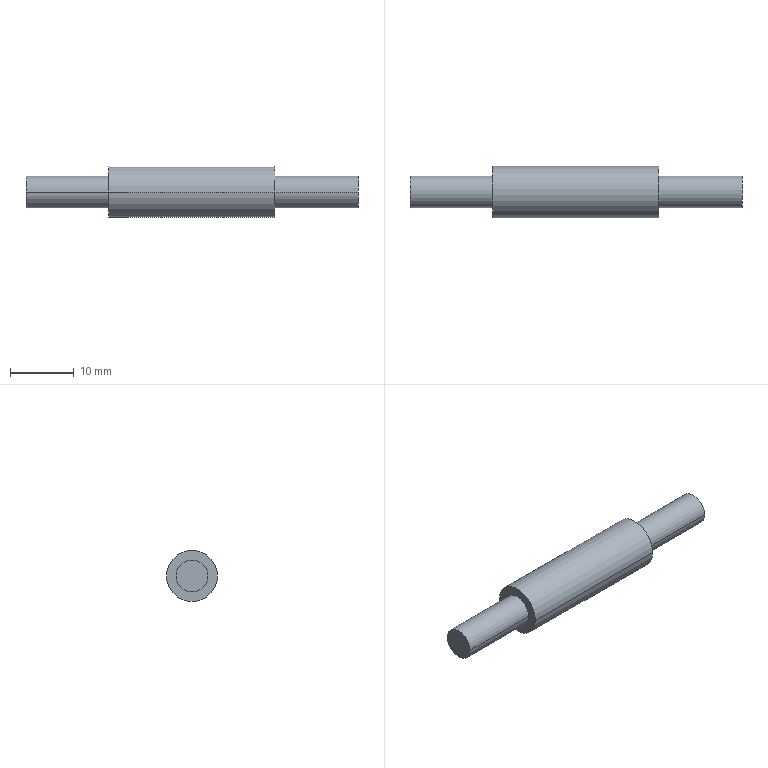Part | SolidWorks | features Revolution 1 | 1 solid | 10 faces | box 52 x 8 x 8 mm | volume 1817 mm3 | cylinder 6 | plane 4 | commonest cylinder face diameters 5 x4 8 x2
STEP:
#1=CARTESIAN_POINT('',(13.,2.5,0.));
#2=VERTEX_POINT('',#1);
#3=CARTESIAN_POINT('',(13.,-2.5,0.));
#4=VERTEX_POINT('',#3);
#5=CARTESIAN_POINT('',(13.,0.,0.));
#6=DIRECTION('',(1.,0.,0.));
#7=DIRECTION('',(0.,1.,0.));
#8=AXIS2_PLACEMENT_3D('',#5,#6,#7);
#9=CIRCLE('',#8,2.5);
#10=EDGE_CURVE('',#2,#4,#9,.T.);
#11=ORIENTED_EDGE('',*,*,#10,.T.);
#12=CARTESIAN_POINT('',(26.,-2.5,0.));
#13=VERTEX_POINT('',#12);
#14=CARTESIAN_POINT('',(26.,-2.5,0.));
#15=DIRECTION('',(1.,0.,0.));
#16=VECTOR('',#15,1000.);
#17=LINE('',#14,#16);
#18=EDGE_CURVE('',#4,#13,#17,.T.);
#19=ORIENTED_EDGE('',*,*,#18,.T.);
#20=CARTESIAN_POINT('',(26.,2.5,0.));
#21=VERTEX_POINT('',#20);
#22=CARTESIAN_POINT('',(26.,0.,0.));
#23=DIRECTION('',(1.,0.,0.));
#24=DIRECTION('',(0.,1.,0.));
#25=AXIS2_PLACEMENT_3D('',#22,#23,#24);
#26=CIRCLE('',#25,2.5);
#27=EDGE_CURVE('',#21,#13,#26,.T.);
#28=ORIENTED_EDGE('',*,*,#27,.F.);
#29=CARTESIAN_POINT('',(26.,2.5,0.));
#30=DIRECTION('',(1.,0.,0.));
#31=VECTOR('',#30,1000.);
#32=LINE('',#29,#31);
#33=EDGE_CURVE('',#2,#21,#32,.T.);
#34=ORIENTED_EDGE('',*,*,#33,.F.);
#35=EDGE_LOOP('',(#11,#19,#28,#34));
#36=FACE_OUTER_BOUND('',#35,.T.);
#37=CARTESIAN_POINT('',(26.,0.,0.));
#38=DIRECTION('',(1.,0.,0.));
#39=DIRECTION('',(0.,1.,0.));
#40=AXIS2_PLACEMENT_3D('',#37,#38,#39);
#41=CYLINDRICAL_SURFACE('',#40,2.5);
#42=ADVANCED_FACE('',(#36),#41,.T.);
#43=CARTESIAN_POINT('',(-13.,4.,0.));
#44=VERTEX_POINT('',#43);
#45=CARTESIAN_POINT('',(-13.,-4.,0.));
#46=VERTEX_POINT('',#45);
#47=CARTESIAN_POINT('',(-13.,0.,0.));
#48=DIRECTION('',(1.,0.,0.));
#49=DIRECTION('',(0.,1.,0.));
#50=AXIS2_PLACEMENT_3D('',#47,#48,#49);
#51=CIRCLE('',#50,4.);
#52=EDGE_CURVE('',#44,#46,#51,.T.);
#53=ORIENTED_EDGE('',*,*,#52,.T.);
#54=CARTESIAN_POINT('',(13.,-4.,0.));
#55=VERTEX_POINT('',#54);
#56=CARTESIAN_POINT('',(26.,-4.,0.));
#57=DIRECTION('',(1.,0.,0.));
#58=VECTOR('',#57,1000.);
#59=LINE('',#56,#58);
#60=EDGE_CURVE('',#46,#55,#59,.T.);
#61=ORIENTED_EDGE('',*,*,#60,.T.);
#62=CARTESIAN_POINT('',(13.,4.,0.));
#63=VERTEX_POINT('',#62);
#64=CARTESIAN_POINT('',(13.,0.,0.));
#65=DIRECTION('',(1.,0.,0.));
#66=DIRECTION('',(0.,1.,0.));
#67=AXIS2_PLACEMENT_3D('',#64,#65,#66);
#68=CIRCLE('',#67,4.);
#69=EDGE_CURVE('',#63,#55,#68,.T.);
#70=ORIENTED_EDGE('',*,*,#69,.F.);
#71=CARTESIAN_POINT('',(26.,4.,0.));
#72=DIRECTION('',(1.,0.,0.));
#73=VECTOR('',#72,1000.);
#74=LINE('',#71,#73);
#75=EDGE_CURVE('',#44,#63,#74,.T.);
#76=ORIENTED_EDGE('',*,*,#75,.F.);
#77=EDGE_LOOP('',(#53,#61,#70,#76));
#78=FACE_OUTER_BOUND('',#77,.T.);
#79=CARTESIAN_POINT('',(26.,0.,0.));
#80=DIRECTION('',(1.,0.,0.));
#81=DIRECTION('',(0.,1.,0.));
#82=AXIS2_PLACEMENT_3D('',#79,#80,#81);
#83=CYLINDRICAL_SURFACE('',#82,4.);
#84=ADVANCED_FACE('',(#78),#83,.T.);
#85=CARTESIAN_POINT('',(-26.,2.5,0.));
#86=VERTEX_POINT('',#85);
#87=CARTESIAN_POINT('',(-26.,-2.5,0.));
#88=VERTEX_POINT('',#87);
#89=CARTESIAN_POINT('',(-26.,0.,0.));
#90=DIRECTION('',(1.,0.,0.));
#91=DIRECTION('',(0.,1.,0.));
#92=AXIS2_PLACEMENT_3D('',#89,#90,#91);
#93=CIRCLE('',#92,2.5);
#94=EDGE_CURVE('',#86,#88,#93,.T.);
#95=ORIENTED_EDGE('',*,*,#94,.T.);
#96=CARTESIAN_POINT('',(-13.,-2.5,0.));
#97=VERTEX_POINT('',#96);
#98=CARTESIAN_POINT('',(26.,-2.5,0.));
#99=DIRECTION('',(1.,0.,0.));
#100=VECTOR('',#99,1000.);
#101=LINE('',#98,#100);
#102=EDGE_CURVE('',#88,#97,#101,.T.);
#103=ORIENTED_EDGE('',*,*,#102,.T.);
#104=CARTESIAN_POINT('',(-13.,2.5,0.));
#105=VERTEX_POINT('',#104);
#106=CARTESIAN_POINT('',(-13.,0.,0.));
#107=DIRECTION('',(1.,0.,0.));
#108=DIRECTION('',(0.,1.,0.));
#109=AXIS2_PLACEMENT_3D('',#106,#107,#108);
#110=CIRCLE('',#109,2.5);
#111=EDGE_CURVE('',#105,#97,#110,.T.);
#112=ORIENTED_EDGE('',*,*,#111,.F.);
#113=CARTESIAN_POINT('',(26.,2.5,0.));
#114=DIRECTION('',(1.,0.,0.));
#115=VECTOR('',#114,1000.);
#116=LINE('',#113,#115);
#117=EDGE_CURVE('',#86,#105,#116,.T.);
#118=ORIENTED_EDGE('',*,*,#117,.F.);
#119=EDGE_LOOP('',(#95,#103,#112,#118));
#120=FACE_OUTER_BOUND('',#119,.T.);
#121=CARTESIAN_POINT('',(26.,0.,0.));
#122=DIRECTION('',(1.,0.,0.));
#123=DIRECTION('',(0.,1.,0.));
#124=AXIS2_PLACEMENT_3D('',#121,#122,#123);
#125=CYLINDRICAL_SURFACE('',#124,2.5);
#126=ADVANCED_FACE('',(#120),#125,.T.);
#127=ORIENTED_EDGE('',*,*,#27,.T.);
#128=CARTESIAN_POINT('',(26.,0.,0.));
#129=DIRECTION('',(1.,0.,0.));
#130=DIRECTION('',(0.,1.,0.));
#131=AXIS2_PLACEMENT_3D('',#128,#129,#130);
#132=CIRCLE('',#131,2.5);
#133=EDGE_CURVE('',#13,#21,#132,.T.);
#134=ORIENTED_EDGE('',*,*,#133,.T.);
#135=EDGE_LOOP('',(#127,#134));
#136=FACE_OUTER_BOUND('',#135,.T.);
#137=CARTESIAN_POINT('',(26.,2.5,0.));
#138=DIRECTION('',(1.,0.,0.));
#139=DIRECTION('',(0.,1.,0.));
#140=AXIS2_PLACEMENT_3D('',#137,#138,#139);
#141=PLANE('',#140);
#142=ADVANCED_FACE('',(#136),#141,.T.);
#143=ORIENTED_EDGE('',*,*,#94,.F.);
#144=CARTESIAN_POINT('',(-26.,0.,0.));
#145=DIRECTION('',(1.,0.,0.));
#146=DIRECTION('',(0.,1.,0.));
#147=AXIS2_PLACEMENT_3D('',#144,#145,#146);
#148=CIRCLE('',#147,2.5);
#149=EDGE_CURVE('',#88,#86,#148,.T.);
#150=ORIENTED_EDGE('',*,*,#149,.F.);
#151=EDGE_LOOP('',(#143,#150));
#152=FACE_OUTER_BOUND('',#151,.T.);
#153=CARTESIAN_POINT('',(-26.,0.,0.));
#154=DIRECTION('',(-1.,0.,0.));
#155=DIRECTION('',(0.,-1.,0.));
#156=AXIS2_PLACEMENT_3D('',#153,#154,#155);
#157=PLANE('',#156);
#158=ADVANCED_FACE('',(#152),#157,.T.);
#159=ORIENTED_EDGE('',*,*,#102,.F.);
#160=ORIENTED_EDGE('',*,*,#149,.T.);
#161=ORIENTED_EDGE('',*,*,#117,.T.);
#162=CARTESIAN_POINT('',(-13.,0.,0.));
#163=DIRECTION('',(1.,0.,0.));
#164=DIRECTION('',(0.,1.,0.));
#165=AXIS2_PLACEMENT_3D('',#162,#163,#164);
#166=CIRCLE('',#165,2.5);
#167=EDGE_CURVE('',#97,#105,#166,.T.);
#168=ORIENTED_EDGE('',*,*,#167,.F.);
#169=EDGE_LOOP('',(#159,#160,#161,#168));
#170=FACE_OUTER_BOUND('',#169,.T.);
#171=CARTESIAN_POINT('',(26.,0.,0.));
#172=DIRECTION('',(1.,0.,0.));
#173=DIRECTION('',(0.,1.,0.));
#174=AXIS2_PLACEMENT_3D('',#171,#172,#173);
#175=CYLINDRICAL_SURFACE('',#174,2.5);
#176=ADVANCED_FACE('',(#170),#175,.T.);
#177=ORIENTED_EDGE('',*,*,#111,.T.);
#178=ORIENTED_EDGE('',*,*,#167,.T.);
#179=EDGE_LOOP('',(#177,#178));
#180=FACE_BOUND('',#179,.T.);
#181=ORIENTED_EDGE('',*,*,#52,.F.);
#182=CARTESIAN_POINT('',(-13.,0.,0.));
#183=DIRECTION('',(1.,0.,0.));
#184=DIRECTION('',(0.,1.,0.));
#185=AXIS2_PLACEMENT_3D('',#182,#183,#184);
#186=CIRCLE('',#185,4.);
#187=EDGE_CURVE('',#46,#44,#186,.T.);
#188=ORIENTED_EDGE('',*,*,#187,.F.);
#189=EDGE_LOOP('',(#181,#188));
#190=FACE_OUTER_BOUND('',#189,.T.);
#191=CARTESIAN_POINT('',(-13.,2.5,0.));
#192=DIRECTION('',(-1.,0.,0.));
#193=DIRECTION('',(0.,-1.,0.));
#194=AXIS2_PLACEMENT_3D('',#191,#192,#193);
#195=PLANE('',#194);
#196=ADVANCED_FACE('',(#180,#190),#195,.T.);
#197=ORIENTED_EDGE('',*,*,#60,.F.);
#198=ORIENTED_EDGE('',*,*,#187,.T.);
#199=ORIENTED_EDGE('',*,*,#75,.T.);
#200=CARTESIAN_POINT('',(13.,0.,0.));
#201=DIRECTION('',(1.,0.,0.));
#202=DIRECTION('',(0.,1.,0.));
#203=AXIS2_PLACEMENT_3D('',#200,#201,#202);
#204=CIRCLE('',#203,4.);
#205=EDGE_CURVE('',#55,#63,#204,.T.);
#206=ORIENTED_EDGE('',*,*,#205,.F.);
#207=EDGE_LOOP('',(#197,#198,#199,#206));
#208=FACE_OUTER_BOUND('',#207,.T.);
#209=CARTESIAN_POINT('',(26.,0.,0.));
#210=DIRECTION('',(1.,0.,0.));
#211=DIRECTION('',(0.,1.,0.));
#212=AXIS2_PLACEMENT_3D('',#209,#210,#211);
#213=CYLINDRICAL_SURFACE('',#212,4.);
#214=ADVANCED_FACE('',(#208),#213,.T.);
#215=ORIENTED_EDGE('',*,*,#69,.T.);
#216=ORIENTED_EDGE('',*,*,#205,.T.);
#217=EDGE_LOOP('',(#215,#216));
#218=FACE_OUTER_BOUND('',#217,.T.);
#219=ORIENTED_EDGE('',*,*,#10,.F.);
#220=CARTESIAN_POINT('',(13.,0.,0.));
#221=DIRECTION('',(1.,0.,0.));
#222=DIRECTION('',(0.,1.,0.));
#223=AXIS2_PLACEMENT_3D('',#220,#221,#222);
#224=CIRCLE('',#223,2.5);
#225=EDGE_CURVE('',#4,#2,#224,.T.);
#226=ORIENTED_EDGE('',*,*,#225,.F.);
#227=EDGE_LOOP('',(#219,#226));
#228=FACE_BOUND('',#227,.T.);
#229=CARTESIAN_POINT('',(13.,4.,0.));
#230=DIRECTION('',(1.,0.,0.));
#231=DIRECTION('',(0.,1.,0.));
#232=AXIS2_PLACEMENT_3D('',#229,#230,#231);
#233=PLANE('',#232);
#234=ADVANCED_FACE('',(#218,#228),#233,.T.);
#235=ORIENTED_EDGE('',*,*,#18,.F.);
#236=ORIENTED_EDGE('',*,*,#225,.T.);
#237=ORIENTED_EDGE('',*,*,#33,.T.);
#238=ORIENTED_EDGE('',*,*,#133,.F.);
#239=EDGE_LOOP('',(#235,#236,#237,#238));
#240=FACE_OUTER_BOUND('',#239,.T.);
#241=CARTESIAN_POINT('',(26.,0.,0.));
#242=DIRECTION('',(1.,0.,0.));
#243=DIRECTION('',(0.,1.,0.));
#244=AXIS2_PLACEMENT_3D('',#241,#242,#243);
#245=CYLINDRICAL_SURFACE('',#244,2.5);
#246=ADVANCED_FACE('',(#240),#245,.T.);
#247=CLOSED_SHELL('',(#42,#84,#126,#142,#158,#176,#196,#214,#234,#246));
#248=MANIFOLD_SOLID_BREP('',#247);
#249=CARTESIAN_POINT('',(0.,0.,0.));
#250=DIRECTION('',(0.,0.,1.));
#251=DIRECTION('',(1.,0.,0.));
#252=AXIS2_PLACEMENT_3D('',#249,#250,#251);
#253=(LENGTH_UNIT()NAMED_UNIT(*)SI_UNIT(.MILLI.,.METRE.));
#254=UNCERTAINTY_MEASURE_WITH_UNIT(LENGTH_MEASURE(0.00001),#253,'','');
#255=(NAMED_UNIT(*)PLANE_ANGLE_UNIT()SI_UNIT($,.RADIAN.));
#256=(NAMED_UNIT(*)SI_UNIT($,.STERADIAN.)SOLID_ANGLE_UNIT());
#257=(GEOMETRIC_REPRESENTATION_CONTEXT(3)GLOBAL_UNCERTAINTY_ASSIGNED_CONTEXT((#254))GLOBAL_UNIT_ASSIGNED_CONTEXT((#253,#255,#256))REPRESENTATION_CONTEXT('',''));
#258=ADVANCED_BREP_SHAPE_REPRESENTATION('',(#248,#252),#257);